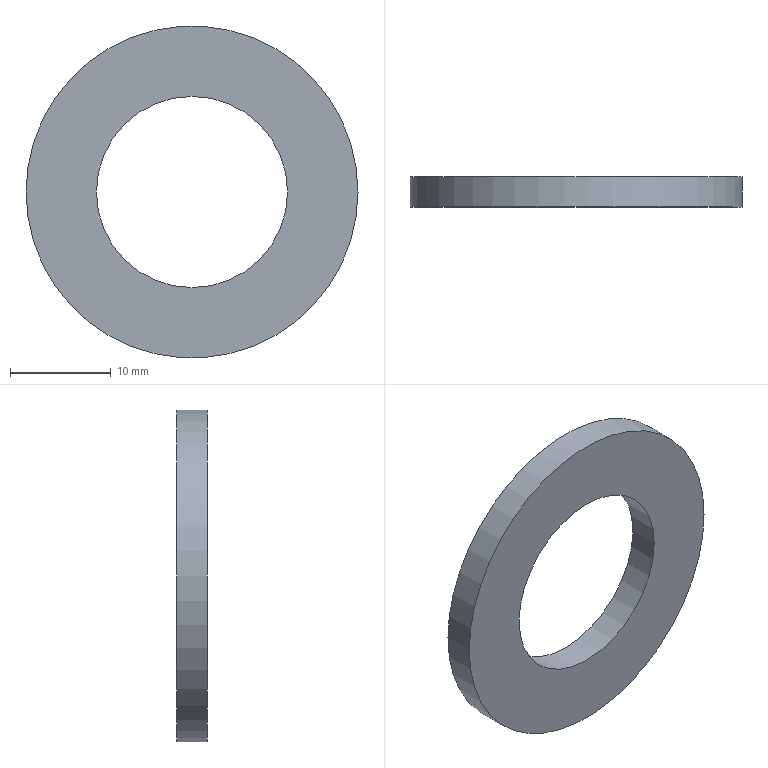Part | NX | features DATUM_CSYS 2, EXTRUDE 1, SKETCH 1 | 1 solid | 4 faces | box 33 x 3 x 33 mm | volume 1715 mm3 | cylinder 2 | plane 2 | commonest cylinder face diameters 19 x1 33 x1
STEP:
#1=CARTESIAN_POINT('',(16.5,-3.,0.));
#2=VERTEX_POINT('',#1);
#3=CARTESIAN_POINT('',(0.,-3.,0.));
#4=DIRECTION('',(0.,-1.,0.));
#5=DIRECTION('',(1.,0.,0.));
#6=AXIS2_PLACEMENT_3D('',#3,#4,#5);
#7=CIRCLE('',#6,16.5);
#8=EDGE_CURVE('',#2,#2,#7,.T.);
#9=ORIENTED_EDGE('',*,*,#8,.F.);
#10=EDGE_LOOP('',(#9));
#11=FACE_BOUND('',#10,.T.);
#12=CARTESIAN_POINT('',(16.5,0.,0.));
#13=VERTEX_POINT('',#12);
#14=CARTESIAN_POINT('',(0.,0.,0.));
#15=DIRECTION('',(0.,-1.,0.));
#16=DIRECTION('',(1.,0.,0.));
#17=AXIS2_PLACEMENT_3D('',#14,#15,#16);
#18=CIRCLE('',#17,16.5);
#19=EDGE_CURVE('',#13,#13,#18,.T.);
#20=ORIENTED_EDGE('',*,*,#19,.T.);
#21=EDGE_LOOP('',(#20));
#22=FACE_BOUND('',#21,.T.);
#23=CARTESIAN_POINT('',(0.,-3.,0.));
#24=DIRECTION('',(0.,1.,0.));
#25=DIRECTION('',(0.,0.,1.));
#26=AXIS2_PLACEMENT_3D('',#23,#24,#25);
#27=CYLINDRICAL_SURFACE('',#26,16.5);
#28=ADVANCED_FACE('',(#11,#22),#27,.T.);
#29=CARTESIAN_POINT('',(9.5,-3.,0.));
#30=VERTEX_POINT('',#29);
#31=CARTESIAN_POINT('',(0.,-3.,0.));
#32=DIRECTION('',(0.,-1.,0.));
#33=DIRECTION('',(1.,0.,0.));
#34=AXIS2_PLACEMENT_3D('',#31,#32,#33);
#35=CIRCLE('',#34,9.5);
#36=EDGE_CURVE('',#30,#30,#35,.T.);
#37=ORIENTED_EDGE('',*,*,#36,.T.);
#38=EDGE_LOOP('',(#37));
#39=FACE_BOUND('',#38,.T.);
#40=CARTESIAN_POINT('',(9.5,0.,0.));
#41=VERTEX_POINT('',#40);
#42=CARTESIAN_POINT('',(0.,0.,0.));
#43=DIRECTION('',(0.,-1.,0.));
#44=DIRECTION('',(1.,0.,0.));
#45=AXIS2_PLACEMENT_3D('',#42,#43,#44);
#46=CIRCLE('',#45,9.5);
#47=EDGE_CURVE('',#41,#41,#46,.T.);
#48=ORIENTED_EDGE('',*,*,#47,.F.);
#49=EDGE_LOOP('',(#48));
#50=FACE_BOUND('',#49,.T.);
#51=CARTESIAN_POINT('',(0.,-3.,0.));
#52=DIRECTION('',(0.,1.,0.));
#53=DIRECTION('',(0.,0.,1.));
#54=AXIS2_PLACEMENT_3D('',#51,#52,#53);
#55=CYLINDRICAL_SURFACE('',#54,9.5);
#56=ADVANCED_FACE('',(#39,#50),#55,.F.);
#57=ORIENTED_EDGE('',*,*,#8,.T.);
#58=EDGE_LOOP('',(#57));
#59=FACE_BOUND('',#58,.T.);
#60=ORIENTED_EDGE('',*,*,#36,.F.);
#61=EDGE_LOOP('',(#60));
#62=FACE_BOUND('',#61,.T.);
#63=CARTESIAN_POINT('',(0.,-3.,0.));
#64=DIRECTION('',(0.,-1.,0.));
#65=DIRECTION('',(0.,0.,-1.));
#66=AXIS2_PLACEMENT_3D('',#63,#64,#65);
#67=PLANE('',#66);
#68=ADVANCED_FACE('',(#59,#62),#67,.T.);
#69=ORIENTED_EDGE('',*,*,#19,.F.);
#70=EDGE_LOOP('',(#69));
#71=FACE_BOUND('',#70,.T.);
#72=ORIENTED_EDGE('',*,*,#47,.T.);
#73=EDGE_LOOP('',(#72));
#74=FACE_BOUND('',#73,.T.);
#75=CARTESIAN_POINT('',(0.,0.,0.));
#76=DIRECTION('',(0.,-1.,0.));
#77=DIRECTION('',(0.,0.,-1.));
#78=AXIS2_PLACEMENT_3D('',#75,#76,#77);
#79=PLANE('',#78);
#80=ADVANCED_FACE('',(#71,#74),#79,.F.);
#81=CLOSED_SHELL('',(#28,#56,#68,#80));
#82=MANIFOLD_SOLID_BREP('',#81);
#83=(LENGTH_UNIT()NAMED_UNIT(*)SI_UNIT(.MILLI.,.METRE.));
#84=UNCERTAINTY_MEASURE_WITH_UNIT(LENGTH_MEASURE(0.00001),#83,'','');
#85=(NAMED_UNIT(*)PLANE_ANGLE_UNIT()SI_UNIT($,.RADIAN.));
#86=(NAMED_UNIT(*)SI_UNIT($,.STERADIAN.)SOLID_ANGLE_UNIT());
#87=(GEOMETRIC_REPRESENTATION_CONTEXT(3)GLOBAL_UNCERTAINTY_ASSIGNED_CONTEXT((#84))GLOBAL_UNIT_ASSIGNED_CONTEXT((#83,#85,#86))REPRESENTATION_CONTEXT('',''));
#88=ADVANCED_BREP_SHAPE_REPRESENTATION('',(#82),#87);